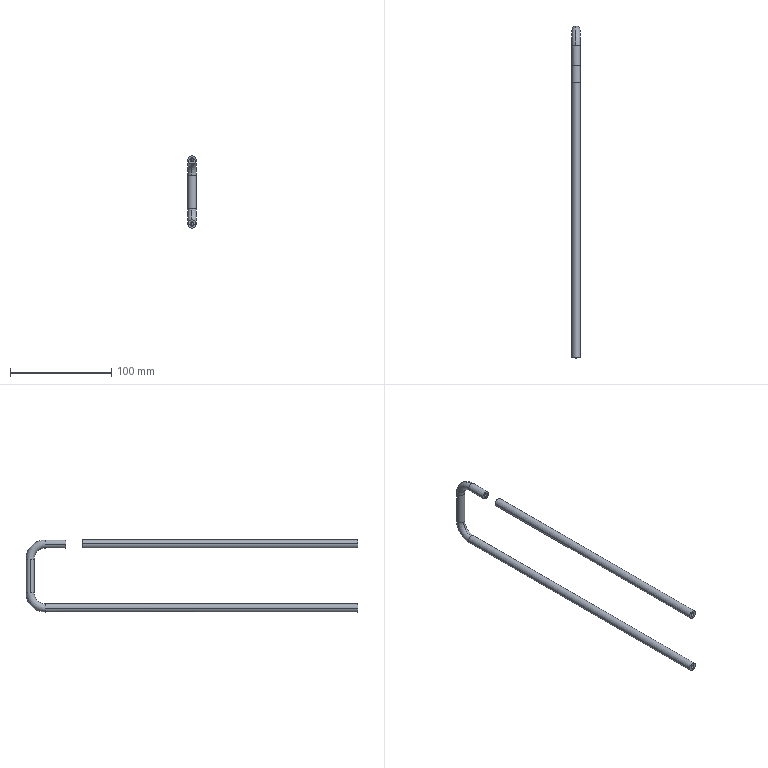Part | SolidWorks | features BaseBody 2 | 2 solids | 28 faces | box 8 x 327.5 x 71.18 mm | volume 25643 mm3 | cylinder 16 | torus 8 | plane 4 | commonest cylinder face diameters 4 x8 8 x8
STEP:
#1=CARTESIAN_POINT('',(168.,-280.,-49.));
#2=VERTEX_POINT('',#1);
#3=CARTESIAN_POINT('',(172.,-280.,-49.));
#4=VERTEX_POINT('',#3);
#5=CARTESIAN_POINT('',(170.,-280.,-49.));
#6=DIRECTION('',(0.,-1.,0.));
#7=DIRECTION('',(-1.,0.,0.));
#8=AXIS2_PLACEMENT_3D('',#5,#6,#7);
#9=CIRCLE('',#8,2.);
#10=EDGE_CURVE('',#2,#4,#9,.T.);
#11=ORIENTED_EDGE('',*,*,#10,.F.);
#12=CARTESIAN_POINT('',(170.,-280.,-49.));
#13=DIRECTION('',(0.,-1.,0.));
#14=DIRECTION('',(1.,0.,0.));
#15=AXIS2_PLACEMENT_3D('',#12,#13,#14);
#16=CIRCLE('',#15,2.);
#17=EDGE_CURVE('',#4,#2,#16,.T.);
#18=ORIENTED_EDGE('',*,*,#17,.F.);
#19=EDGE_LOOP('',(#11,#18));
#20=FACE_BOUND('',#19,.T.);
#21=CARTESIAN_POINT('',(166.,-280.,-49.));
#22=VERTEX_POINT('',#21);
#23=CARTESIAN_POINT('',(174.,-280.,-49.));
#24=VERTEX_POINT('',#23);
#25=CARTESIAN_POINT('',(170.,-280.,-49.));
#26=DIRECTION('',(0.,1.,0.));
#27=DIRECTION('',(-1.,0.,0.));
#28=AXIS2_PLACEMENT_3D('',#25,#26,#27);
#29=CIRCLE('',#28,4.);
#30=EDGE_CURVE('',#22,#24,#29,.T.);
#31=ORIENTED_EDGE('',*,*,#30,.F.);
#32=CARTESIAN_POINT('',(170.,-280.,-49.));
#33=DIRECTION('',(0.,1.,0.));
#34=DIRECTION('',(1.,0.,0.));
#35=AXIS2_PLACEMENT_3D('',#32,#33,#34);
#36=CIRCLE('',#35,4.);
#37=EDGE_CURVE('',#24,#22,#36,.T.);
#38=ORIENTED_EDGE('',*,*,#37,.F.);
#39=EDGE_LOOP('',(#31,#38));
#40=FACE_OUTER_BOUND('',#39,.T.);
#41=CARTESIAN_POINT('',(170.,-280.,-49.));
#42=DIRECTION('',(0.,-1.,0.));
#43=DIRECTION('',(0.,0.,-1.));
#44=AXIS2_PLACEMENT_3D('',#41,#42,#43);
#45=PLANE('',#44);
#46=ADVANCED_FACE('',(#20,#40),#45,.T.);
#47=CARTESIAN_POINT('',(168.,8.5,14.08));
#48=VERTEX_POINT('',#47);
#49=CARTESIAN_POINT('',(172.,8.5,14.08));
#50=VERTEX_POINT('',#49);
#51=CARTESIAN_POINT('',(170.,8.5,14.08));
#52=DIRECTION('',(0.,-1.,0.));
#53=DIRECTION('',(-1.,0.,0.));
#54=AXIS2_PLACEMENT_3D('',#51,#52,#53);
#55=CIRCLE('',#54,2.);
#56=EDGE_CURVE('',#48,#50,#55,.T.);
#57=ORIENTED_EDGE('',*,*,#56,.F.);
#58=CARTESIAN_POINT('',(170.,8.5,14.08));
#59=DIRECTION('',(0.,-1.,0.));
#60=DIRECTION('',(1.,0.,0.));
#61=AXIS2_PLACEMENT_3D('',#58,#59,#60);
#62=CIRCLE('',#61,2.);
#63=EDGE_CURVE('',#50,#48,#62,.T.);
#64=ORIENTED_EDGE('',*,*,#63,.F.);
#65=EDGE_LOOP('',(#57,#64));
#66=FACE_BOUND('',#65,.T.);
#67=CARTESIAN_POINT('',(166.,8.5,14.08));
#68=VERTEX_POINT('',#67);
#69=CARTESIAN_POINT('',(174.,8.5,14.08));
#70=VERTEX_POINT('',#69);
#71=CARTESIAN_POINT('',(170.,8.5,14.08));
#72=DIRECTION('',(0.,1.,0.));
#73=DIRECTION('',(-1.,0.,0.));
#74=AXIS2_PLACEMENT_3D('',#71,#72,#73);
#75=CIRCLE('',#74,4.);
#76=EDGE_CURVE('',#68,#70,#75,.T.);
#77=ORIENTED_EDGE('',*,*,#76,.F.);
#78=CARTESIAN_POINT('',(170.,8.5,14.08));
#79=DIRECTION('',(0.,1.,0.));
#80=DIRECTION('',(1.,0.,0.));
#81=AXIS2_PLACEMENT_3D('',#78,#79,#80);
#82=CIRCLE('',#81,4.);
#83=EDGE_CURVE('',#70,#68,#82,.T.);
#84=ORIENTED_EDGE('',*,*,#83,.F.);
#85=EDGE_LOOP('',(#77,#84));
#86=FACE_OUTER_BOUND('',#85,.T.);
#87=CARTESIAN_POINT('',(170.,8.5,14.08));
#88=DIRECTION('',(0.,-1.,0.));
#89=DIRECTION('',(0.,0.,-1.));
#90=AXIS2_PLACEMENT_3D('',#87,#88,#89);
#91=PLANE('',#90);
#92=ADVANCED_FACE('',(#66,#86),#91,.T.);
#93=CARTESIAN_POINT('',(166.,28.5,-49.));
#94=VERTEX_POINT('',#93);
#95=CARTESIAN_POINT('',(170.,28.5,-45.));
#96=VERTEX_POINT('',#95);
#97=CARTESIAN_POINT('',(170.,28.5,-49.));
#98=DIRECTION('',(0.,1.,0.));
#99=DIRECTION('',(-1.,0.,0.));
#100=AXIS2_PLACEMENT_3D('',#97,#98,#99);
#101=CIRCLE('',#100,4.);
#102=EDGE_CURVE('',#94,#96,#101,.T.);
#103=ORIENTED_EDGE('',*,*,#102,.F.);
#104=CARTESIAN_POINT('',(166.,-280.,-49.));
#105=DIRECTION('',(0.,1.,0.));
#106=VECTOR('',#105,1000.);
#107=LINE('',#104,#106);
#108=EDGE_CURVE('',#22,#94,#107,.T.);
#109=ORIENTED_EDGE('',*,*,#108,.F.);
#110=ORIENTED_EDGE('',*,*,#30,.T.);
#111=CARTESIAN_POINT('',(174.,28.5,-49.));
#112=VERTEX_POINT('',#111);
#113=CARTESIAN_POINT('',(174.,28.5,-49.));
#114=DIRECTION('',(0.,-1.,0.));
#115=VECTOR('',#114,1000.);
#116=LINE('',#113,#115);
#117=EDGE_CURVE('',#112,#24,#116,.T.);
#118=ORIENTED_EDGE('',*,*,#117,.F.);
#119=CARTESIAN_POINT('',(170.,28.5,-49.));
#120=DIRECTION('',(0.,1.,0.));
#121=DIRECTION('',(0.,0.,1.));
#122=AXIS2_PLACEMENT_3D('',#119,#120,#121);
#123=CIRCLE('',#122,4.);
#124=EDGE_CURVE('',#96,#112,#123,.T.);
#125=ORIENTED_EDGE('',*,*,#124,.F.);
#126=EDGE_LOOP('',(#103,#109,#110,#118,#125));
#127=FACE_OUTER_BOUND('',#126,.T.);
#128=CARTESIAN_POINT('',(170.,-280.,-49.));
#129=DIRECTION('',(0.,1.,0.));
#130=DIRECTION('',(-1.,0.,0.));
#131=AXIS2_PLACEMENT_3D('',#128,#129,#130);
#132=CYLINDRICAL_SURFACE('',#131,4.);
#133=ADVANCED_FACE('',(#127),#132,.T.);
#134=ORIENTED_EDGE('',*,*,#117,.T.);
#135=ORIENTED_EDGE('',*,*,#37,.T.);
#136=ORIENTED_EDGE('',*,*,#108,.T.);
#137=CARTESIAN_POINT('',(170.,28.5,-53.));
#138=VERTEX_POINT('',#137);
#139=CARTESIAN_POINT('',(170.,28.5,-49.));
#140=DIRECTION('',(0.,1.,0.));
#141=DIRECTION('',(0.,0.,-1.));
#142=AXIS2_PLACEMENT_3D('',#139,#140,#141);
#143=CIRCLE('',#142,4.);
#144=EDGE_CURVE('',#138,#94,#143,.T.);
#145=ORIENTED_EDGE('',*,*,#144,.F.);
#146=CARTESIAN_POINT('',(170.,28.5,-49.));
#147=DIRECTION('',(0.,-1.,0.));
#148=DIRECTION('',(0.,0.,-1.));
#149=AXIS2_PLACEMENT_3D('',#146,#147,#148);
#150=CIRCLE('',#149,4.);
#151=EDGE_CURVE('',#138,#112,#150,.T.);
#152=ORIENTED_EDGE('',*,*,#151,.T.);
#153=EDGE_LOOP('',(#134,#135,#136,#145,#152));
#154=FACE_OUTER_BOUND('',#153,.T.);
#155=CARTESIAN_POINT('',(170.,-280.,-49.));
#156=DIRECTION('',(0.,1.,0.));
#157=DIRECTION('',(-1.,0.,0.));
#158=AXIS2_PLACEMENT_3D('',#155,#156,#157);
#159=CYLINDRICAL_SURFACE('',#158,4.);
#160=ADVANCED_FACE('',(#154),#159,.T.);
#161=CARTESIAN_POINT('',(170.,39.5,-34.));
#162=VERTEX_POINT('',#161);
#163=CARTESIAN_POINT('',(166.,43.5,-34.));
#164=VERTEX_POINT('',#163);
#165=CARTESIAN_POINT('',(170.,43.5,-34.));
#166=DIRECTION('',(0.,0.,-1.));
#167=DIRECTION('',(0.,-1.,0.));
#168=AXIS2_PLACEMENT_3D('',#165,#166,#167);
#169=CIRCLE('',#168,4.);
#170=EDGE_CURVE('',#162,#164,#169,.T.);
#171=ORIENTED_EDGE('',*,*,#170,.T.);
#172=CARTESIAN_POINT('',(170.,47.5,-34.));
#173=VERTEX_POINT('',#172);
#174=CARTESIAN_POINT('',(170.,43.5,-34.));
#175=DIRECTION('',(0.,0.,-1.));
#176=DIRECTION('',(-1.,0.,0.));
#177=AXIS2_PLACEMENT_3D('',#174,#175,#176);
#178=CIRCLE('',#177,4.);
#179=EDGE_CURVE('',#164,#173,#178,.T.);
#180=ORIENTED_EDGE('',*,*,#179,.T.);
#181=CARTESIAN_POINT('',(170.,28.5,-34.));
#182=DIRECTION('',(1.,0.,0.));
#183=DIRECTION('',(0.,0.,-1.));
#184=AXIS2_PLACEMENT_3D('',#181,#182,#183);
#185=CIRCLE('',#184,19.);
#186=EDGE_CURVE('',#138,#173,#185,.T.);
#187=ORIENTED_EDGE('',*,*,#186,.F.);
#188=ORIENTED_EDGE('',*,*,#144,.T.);
#189=ORIENTED_EDGE('',*,*,#102,.T.);
#190=CARTESIAN_POINT('',(170.,28.5,-34.));
#191=DIRECTION('',(-1.,0.,0.));
#192=DIRECTION('',(0.,1.,0.));
#193=AXIS2_PLACEMENT_3D('',#190,#191,#192);
#194=CIRCLE('',#193,11.);
#195=EDGE_CURVE('',#162,#96,#194,.T.);
#196=ORIENTED_EDGE('',*,*,#195,.F.);
#197=EDGE_LOOP('',(#171,#180,#187,#188,#189,#196));
#198=FACE_OUTER_BOUND('',#197,.T.);
#199=CARTESIAN_POINT('',(170.,28.5,-34.));
#200=DIRECTION('',(-1.,0.,0.));
#201=DIRECTION('',(0.,0.,-1.));
#202=AXIS2_PLACEMENT_3D('',#199,#200,#201);
#203=TOROIDAL_SURFACE('',#202,15.,4.);
#204=ADVANCED_FACE('',(#198),#203,.T.);
#205=CARTESIAN_POINT('',(174.,43.5,-34.));
#206=VERTEX_POINT('',#205);
#207=CARTESIAN_POINT('',(170.,43.5,-34.));
#208=DIRECTION('',(0.,0.,1.));
#209=DIRECTION('',(0.,-1.,0.));
#210=AXIS2_PLACEMENT_3D('',#207,#208,#209);
#211=CIRCLE('',#210,4.);
#212=EDGE_CURVE('',#162,#206,#211,.T.);
#213=ORIENTED_EDGE('',*,*,#212,.F.);
#214=ORIENTED_EDGE('',*,*,#195,.T.);
#215=ORIENTED_EDGE('',*,*,#124,.T.);
#216=ORIENTED_EDGE('',*,*,#151,.F.);
#217=ORIENTED_EDGE('',*,*,#186,.T.);
#218=CARTESIAN_POINT('',(170.,43.5,-34.));
#219=DIRECTION('',(0.,0.,1.));
#220=DIRECTION('',(1.,0.,0.));
#221=AXIS2_PLACEMENT_3D('',#218,#219,#220);
#222=CIRCLE('',#221,4.);
#223=EDGE_CURVE('',#206,#173,#222,.T.);
#224=ORIENTED_EDGE('',*,*,#223,.F.);
#225=EDGE_LOOP('',(#213,#214,#215,#216,#217,#224));
#226=FACE_OUTER_BOUND('',#225,.T.);
#227=CARTESIAN_POINT('',(170.,28.5,-34.));
#228=DIRECTION('',(-1.,0.,0.));
#229=DIRECTION('',(0.,0.,-1.));
#230=AXIS2_PLACEMENT_3D('',#227,#228,#229);
#231=TOROIDAL_SURFACE('',#230,15.,4.);
#232=ADVANCED_FACE('',(#226),#231,.T.);
#233=CARTESIAN_POINT('',(166.,43.5,-0.92));
#234=VERTEX_POINT('',#233);
#235=CARTESIAN_POINT('',(170.,39.5,-0.92));
#236=VERTEX_POINT('',#235);
#237=CARTESIAN_POINT('',(170.,43.5,-0.92));
#238=DIRECTION('',(0.,0.,1.));
#239=DIRECTION('',(-1.,0.,0.));
#240=AXIS2_PLACEMENT_3D('',#237,#238,#239);
#241=CIRCLE('',#240,4.);
#242=EDGE_CURVE('',#234,#236,#241,.T.);
#243=ORIENTED_EDGE('',*,*,#242,.F.);
#244=CARTESIAN_POINT('',(166.,43.5,-34.));
#245=DIRECTION('',(0.,0.,1.));
#246=VECTOR('',#245,1000.);
#247=LINE('',#244,#246);
#248=EDGE_CURVE('',#164,#234,#247,.T.);
#249=ORIENTED_EDGE('',*,*,#248,.F.);
#250=ORIENTED_EDGE('',*,*,#170,.F.);
#251=ORIENTED_EDGE('',*,*,#212,.T.);
#252=CARTESIAN_POINT('',(174.,43.5,-0.92));
#253=VERTEX_POINT('',#252);
#254=CARTESIAN_POINT('',(174.,43.5,-0.92));
#255=DIRECTION('',(0.,0.,-1.));
#256=VECTOR('',#255,1000.);
#257=LINE('',#254,#256);
#258=EDGE_CURVE('',#253,#206,#257,.T.);
#259=ORIENTED_EDGE('',*,*,#258,.F.);
#260=CARTESIAN_POINT('',(170.,43.5,-0.92));
#261=DIRECTION('',(0.,0.,1.));
#262=DIRECTION('',(0.,-1.,0.));
#263=AXIS2_PLACEMENT_3D('',#260,#261,#262);
#264=CIRCLE('',#263,4.);
#265=EDGE_CURVE('',#236,#253,#264,.T.);
#266=ORIENTED_EDGE('',*,*,#265,.F.);
#267=EDGE_LOOP('',(#243,#249,#250,#251,#259,#266));
#268=FACE_OUTER_BOUND('',#267,.T.);
#269=CARTESIAN_POINT('',(170.,43.5,-34.));
#270=DIRECTION('',(0.,0.,1.));
#271=DIRECTION('',(-1.,0.,0.));
#272=AXIS2_PLACEMENT_3D('',#269,#270,#271);
#273=CYLINDRICAL_SURFACE('',#272,4.);
#274=ADVANCED_FACE('',(#268),#273,.T.);
#275=ORIENTED_EDGE('',*,*,#258,.T.);
#276=ORIENTED_EDGE('',*,*,#223,.T.);
#277=ORIENTED_EDGE('',*,*,#179,.F.);
#278=ORIENTED_EDGE('',*,*,#248,.T.);
#279=CARTESIAN_POINT('',(170.,47.5,-0.92));
#280=VERTEX_POINT('',#279);
#281=CARTESIAN_POINT('',(170.,43.5,-0.92));
#282=DIRECTION('',(0.,0.,1.));
#283=DIRECTION('',(0.,1.,0.));
#284=AXIS2_PLACEMENT_3D('',#281,#282,#283);
#285=CIRCLE('',#284,4.);
#286=EDGE_CURVE('',#280,#234,#285,.T.);
#287=ORIENTED_EDGE('',*,*,#286,.F.);
#288=CARTESIAN_POINT('',(170.,43.5,-0.92));
#289=DIRECTION('',(0.,0.,-1.));
#290=DIRECTION('',(0.,1.,0.));
#291=AXIS2_PLACEMENT_3D('',#288,#289,#290);
#292=CIRCLE('',#291,4.);
#293=EDGE_CURVE('',#280,#253,#292,.T.);
#294=ORIENTED_EDGE('',*,*,#293,.T.);
#295=EDGE_LOOP('',(#275,#276,#277,#278,#287,#294));
#296=FACE_OUTER_BOUND('',#295,.T.);
#297=CARTESIAN_POINT('',(170.,43.5,-34.));
#298=DIRECTION('',(0.,0.,1.));
#299=DIRECTION('',(-1.,0.,0.));
#300=AXIS2_PLACEMENT_3D('',#297,#298,#299);
#301=CYLINDRICAL_SURFACE('',#300,4.);
#302=ADVANCED_FACE('',(#296),#301,.T.);
#303=CARTESIAN_POINT('',(170.,28.5,10.08));
#304=VERTEX_POINT('',#303);
#305=CARTESIAN_POINT('',(166.,28.5,14.08));
#306=VERTEX_POINT('',#305);
#307=CARTESIAN_POINT('',(170.,28.5,14.08));
#308=DIRECTION('',(0.,1.,0.));
#309=DIRECTION('',(0.,0.,-1.));
#310=AXIS2_PLACEMENT_3D('',#307,#308,#309);
#311=CIRCLE('',#310,4.);
#312=EDGE_CURVE('',#304,#306,#311,.T.);
#313=ORIENTED_EDGE('',*,*,#312,.T.);
#314=CARTESIAN_POINT('',(170.,28.5,18.08));
#315=VERTEX_POINT('',#314);
#316=CARTESIAN_POINT('',(170.,28.5,14.08));
#317=DIRECTION('',(0.,1.,0.));
#318=DIRECTION('',(-1.,0.,0.));
#319=AXIS2_PLACEMENT_3D('',#316,#317,#318);
#320=CIRCLE('',#319,4.);
#321=EDGE_CURVE('',#306,#315,#320,.T.);
#322=ORIENTED_EDGE('',*,*,#321,.T.);
#323=CARTESIAN_POINT('',(170.,28.5,-0.92));
#324=DIRECTION('',(1.,0.,0.));
#325=DIRECTION('',(0.,1.,0.));
#326=AXIS2_PLACEMENT_3D('',#323,#324,#325);
#327=CIRCLE('',#326,19.);
#328=EDGE_CURVE('',#280,#315,#327,.T.);
#329=ORIENTED_EDGE('',*,*,#328,.F.);
#330=ORIENTED_EDGE('',*,*,#286,.T.);
#331=ORIENTED_EDGE('',*,*,#242,.T.);
#332=CARTESIAN_POINT('',(170.,28.5,-0.92));
#333=DIRECTION('',(-1.,0.,0.));
#334=DIRECTION('',(0.,0.,1.));
#335=AXIS2_PLACEMENT_3D('',#332,#333,#334);
#336=CIRCLE('',#335,11.);
#337=EDGE_CURVE('',#304,#236,#336,.T.);
#338=ORIENTED_EDGE('',*,*,#337,.F.);
#339=EDGE_LOOP('',(#313,#322,#329,#330,#331,#338));
#340=FACE_OUTER_BOUND('',#339,.T.);
#341=CARTESIAN_POINT('',(170.,28.5,-0.92));
#342=DIRECTION('',(-1.,0.,0.));
#343=DIRECTION('',(0.,1.,0.));
#344=AXIS2_PLACEMENT_3D('',#341,#342,#343);
#345=TOROIDAL_SURFACE('',#344,15.,4.);
#346=ADVANCED_FACE('',(#340),#345,.T.);
#347=CARTESIAN_POINT('',(174.,28.5,14.08));
#348=VERTEX_POINT('',#347);
#349=CARTESIAN_POINT('',(170.,28.5,14.08));
#350=DIRECTION('',(0.,-1.,0.));
#351=DIRECTION('',(0.,0.,-1.));
#352=AXIS2_PLACEMENT_3D('',#349,#350,#351);
#353=CIRCLE('',#352,4.);
#354=EDGE_CURVE('',#304,#348,#353,.T.);
#355=ORIENTED_EDGE('',*,*,#354,.F.);
#356=ORIENTED_EDGE('',*,*,#337,.T.);
#357=ORIENTED_EDGE('',*,*,#265,.T.);
#358=ORIENTED_EDGE('',*,*,#293,.F.);
#359=ORIENTED_EDGE('',*,*,#328,.T.);
#360=CARTESIAN_POINT('',(170.,28.5,14.08));
#361=DIRECTION('',(0.,-1.,0.));
#362=DIRECTION('',(1.,0.,0.));
#363=AXIS2_PLACEMENT_3D('',#360,#361,#362);
#364=CIRCLE('',#363,4.);
#365=EDGE_CURVE('',#348,#315,#364,.T.);
#366=ORIENTED_EDGE('',*,*,#365,.F.);
#367=EDGE_LOOP('',(#355,#356,#357,#358,#359,#366));
#368=FACE_OUTER_BOUND('',#367,.T.);
#369=CARTESIAN_POINT('',(170.,28.5,-0.92));
#370=DIRECTION('',(-1.,0.,0.));
#371=DIRECTION('',(0.,1.,0.));
#372=AXIS2_PLACEMENT_3D('',#369,#370,#371);
#373=TOROIDAL_SURFACE('',#372,15.,4.);
#374=ADVANCED_FACE('',(#368),#373,.T.);
#375=ORIENTED_EDGE('',*,*,#83,.T.);
#376=CARTESIAN_POINT('',(166.,28.5,14.08));
#377=DIRECTION('',(0.,-1.,0.));
#378=VECTOR('',#377,1000.);
#379=LINE('',#376,#378);
#380=EDGE_CURVE('',#306,#68,#379,.T.);
#381=ORIENTED_EDGE('',*,*,#380,.F.);
#382=ORIENTED_EDGE('',*,*,#312,.F.);
#383=ORIENTED_EDGE('',*,*,#354,.T.);
#384=CARTESIAN_POINT('',(174.,8.5,14.08));
#385=DIRECTION('',(0.,1.,0.));
#386=VECTOR('',#385,1000.);
#387=LINE('',#384,#386);
#388=EDGE_CURVE('',#70,#348,#387,.T.);
#389=ORIENTED_EDGE('',*,*,#388,.F.);
#390=EDGE_LOOP('',(#375,#381,#382,#383,#389));
#391=FACE_OUTER_BOUND('',#390,.T.);
#392=CARTESIAN_POINT('',(170.,28.5,14.08));
#393=DIRECTION('',(0.,-1.,0.));
#394=DIRECTION('',(-1.,0.,0.));
#395=AXIS2_PLACEMENT_3D('',#392,#393,#394);
#396=CYLINDRICAL_SURFACE('',#395,4.);
#397=ADVANCED_FACE('',(#391),#396,.T.);
#398=ORIENTED_EDGE('',*,*,#388,.T.);
#399=ORIENTED_EDGE('',*,*,#365,.T.);
#400=ORIENTED_EDGE('',*,*,#321,.F.);
#401=ORIENTED_EDGE('',*,*,#380,.T.);
#402=ORIENTED_EDGE('',*,*,#76,.T.);
#403=EDGE_LOOP('',(#398,#399,#400,#401,#402));
#404=FACE_OUTER_BOUND('',#403,.T.);
#405=CARTESIAN_POINT('',(170.,28.5,14.08));
#406=DIRECTION('',(0.,-1.,0.));
#407=DIRECTION('',(-1.,0.,0.));
#408=AXIS2_PLACEMENT_3D('',#405,#406,#407);
#409=CYLINDRICAL_SURFACE('',#408,4.);
#410=ADVANCED_FACE('',(#404),#409,.T.);
#411=ORIENTED_EDGE('',*,*,#17,.T.);
#412=CARTESIAN_POINT('',(168.,28.5,-49.));
#413=VERTEX_POINT('',#412);
#414=CARTESIAN_POINT('',(168.,28.5,-49.));
#415=DIRECTION('',(0.,-1.,0.));
#416=VECTOR('',#415,1000.);
#417=LINE('',#414,#416);
#418=EDGE_CURVE('',#413,#2,#417,.T.);
#419=ORIENTED_EDGE('',*,*,#418,.F.);
#420=CARTESIAN_POINT('',(170.,28.5,-47.));
#421=VERTEX_POINT('',#420);
#422=CARTESIAN_POINT('',(170.,28.5,-49.));
#423=DIRECTION('',(0.,-1.,0.));
#424=DIRECTION('',(0.,0.,1.));
#425=AXIS2_PLACEMENT_3D('',#422,#423,#424);
#426=CIRCLE('',#425,2.);
#427=EDGE_CURVE('',#421,#413,#426,.T.);
#428=ORIENTED_EDGE('',*,*,#427,.F.);
#429=CARTESIAN_POINT('',(172.,28.5,-49.));
#430=VERTEX_POINT('',#429);
#431=CARTESIAN_POINT('',(170.,28.5,-49.));
#432=DIRECTION('',(0.,-1.,0.));
#433=DIRECTION('',(1.,0.,0.));
#434=AXIS2_PLACEMENT_3D('',#431,#432,#433);
#435=CIRCLE('',#434,2.);
#436=EDGE_CURVE('',#430,#421,#435,.T.);
#437=ORIENTED_EDGE('',*,*,#436,.F.);
#438=CARTESIAN_POINT('',(172.,-280.,-49.));
#439=DIRECTION('',(0.,1.,0.));
#440=VECTOR('',#439,1000.);
#441=LINE('',#438,#440);
#442=EDGE_CURVE('',#4,#430,#441,.T.);
#443=ORIENTED_EDGE('',*,*,#442,.F.);
#444=EDGE_LOOP('',(#411,#419,#428,#437,#443));
#445=FACE_OUTER_BOUND('',#444,.T.);
#446=CARTESIAN_POINT('',(170.,-280.,-49.));
#447=DIRECTION('',(0.,1.,0.));
#448=DIRECTION('',(-1.,0.,0.));
#449=AXIS2_PLACEMENT_3D('',#446,#447,#448);
#450=CYLINDRICAL_SURFACE('',#449,2.);
#451=ADVANCED_FACE('',(#445),#450,.F.);
#452=ORIENTED_EDGE('',*,*,#442,.T.);
#453=CARTESIAN_POINT('',(170.,28.5,-51.));
#454=VERTEX_POINT('',#453);
#455=CARTESIAN_POINT('',(170.,28.5,-49.));
#456=DIRECTION('',(0.,1.,0.));
#457=DIRECTION('',(1.,0.,0.));
#458=AXIS2_PLACEMENT_3D('',#455,#456,#457);
#459=CIRCLE('',#458,2.);
#460=EDGE_CURVE('',#430,#454,#459,.T.);
#461=ORIENTED_EDGE('',*,*,#460,.T.);
#462=CARTESIAN_POINT('',(170.,28.5,-49.));
#463=DIRECTION('',(0.,1.,0.));
#464=DIRECTION('',(0.,0.,-1.));
#465=AXIS2_PLACEMENT_3D('',#462,#463,#464);
#466=CIRCLE('',#465,2.);
#467=EDGE_CURVE('',#454,#413,#466,.T.);
#468=ORIENTED_EDGE('',*,*,#467,.T.);
#469=ORIENTED_EDGE('',*,*,#418,.T.);
#470=ORIENTED_EDGE('',*,*,#10,.T.);
#471=EDGE_LOOP('',(#452,#461,#468,#469,#470));
#472=FACE_OUTER_BOUND('',#471,.T.);
#473=CARTESIAN_POINT('',(170.,-280.,-49.));
#474=DIRECTION('',(0.,1.,0.));
#475=DIRECTION('',(-1.,0.,0.));
#476=AXIS2_PLACEMENT_3D('',#473,#474,#475);
#477=CYLINDRICAL_SURFACE('',#476,2.);
#478=ADVANCED_FACE('',(#472),#477,.F.);
#479=ORIENTED_EDGE('',*,*,#427,.T.);
#480=ORIENTED_EDGE('',*,*,#467,.F.);
#481=CARTESIAN_POINT('',(170.,45.5,-34.));
#482=VERTEX_POINT('',#481);
#483=CARTESIAN_POINT('',(170.,28.5,-34.));
#484=DIRECTION('',(-1.,0.,0.));
#485=DIRECTION('',(0.,1.,0.));
#486=AXIS2_PLACEMENT_3D('',#483,#484,#485);
#487=CIRCLE('',#486,17.);
#488=EDGE_CURVE('',#482,#454,#487,.T.);
#489=ORIENTED_EDGE('',*,*,#488,.F.);
#490=CARTESIAN_POINT('',(168.,43.5,-34.));
#491=VERTEX_POINT('',#490);
#492=CARTESIAN_POINT('',(170.,43.5,-34.));
#493=DIRECTION('',(0.,0.,-1.));
#494=DIRECTION('',(-1.,0.,0.));
#495=AXIS2_PLACEMENT_3D('',#492,#493,#494);
#496=CIRCLE('',#495,2.);
#497=EDGE_CURVE('',#491,#482,#496,.T.);
#498=ORIENTED_EDGE('',*,*,#497,.F.);
#499=CARTESIAN_POINT('',(170.,41.5,-34.));
#500=VERTEX_POINT('',#499);
#501=CARTESIAN_POINT('',(170.,43.5,-34.));
#502=DIRECTION('',(0.,0.,1.));
#503=DIRECTION('',(-1.,0.,0.));
#504=AXIS2_PLACEMENT_3D('',#501,#502,#503);
#505=CIRCLE('',#504,2.);
#506=EDGE_CURVE('',#491,#500,#505,.T.);
#507=ORIENTED_EDGE('',*,*,#506,.T.);
#508=CARTESIAN_POINT('',(170.,28.5,-34.));
#509=DIRECTION('',(1.,0.,0.));
#510=DIRECTION('',(0.,0.,-1.));
#511=AXIS2_PLACEMENT_3D('',#508,#509,#510);
#512=CIRCLE('',#511,13.);
#513=EDGE_CURVE('',#421,#500,#512,.T.);
#514=ORIENTED_EDGE('',*,*,#513,.F.);
#515=EDGE_LOOP('',(#479,#480,#489,#498,#507,#514));
#516=FACE_OUTER_BOUND('',#515,.T.);
#517=CARTESIAN_POINT('',(170.,28.5,-34.));
#518=DIRECTION('',(1.,0.,0.));
#519=DIRECTION('',(0.,1.,0.));
#520=AXIS2_PLACEMENT_3D('',#517,#518,#519);
#521=TOROIDAL_SURFACE('',#520,15.,2.);
#522=ADVANCED_FACE('',(#516),#521,.F.);
#523=ORIENTED_EDGE('',*,*,#436,.T.);
#524=ORIENTED_EDGE('',*,*,#513,.T.);
#525=CARTESIAN_POINT('',(172.,43.5,-34.));
#526=VERTEX_POINT('',#525);
#527=CARTESIAN_POINT('',(170.,43.5,-34.));
#528=DIRECTION('',(0.,0.,-1.));
#529=DIRECTION('',(1.,0.,0.));
#530=AXIS2_PLACEMENT_3D('',#527,#528,#529);
#531=CIRCLE('',#530,2.);
#532=EDGE_CURVE('',#526,#500,#531,.T.);
#533=ORIENTED_EDGE('',*,*,#532,.F.);
#534=CARTESIAN_POINT('',(170.,43.5,-34.));
#535=DIRECTION('',(0.,0.,-1.));
#536=DIRECTION('',(0.,1.,0.));
#537=AXIS2_PLACEMENT_3D('',#534,#535,#536);
#538=CIRCLE('',#537,2.);
#539=EDGE_CURVE('',#482,#526,#538,.T.);
#540=ORIENTED_EDGE('',*,*,#539,.F.);
#541=ORIENTED_EDGE('',*,*,#488,.T.);
#542=ORIENTED_EDGE('',*,*,#460,.F.);
#543=EDGE_LOOP('',(#523,#524,#533,#540,#541,#542));
#544=FACE_OUTER_BOUND('',#543,.T.);
#545=CARTESIAN_POINT('',(170.,28.5,-34.));
#546=DIRECTION('',(1.,0.,0.));
#547=DIRECTION('',(0.,1.,0.));
#548=AXIS2_PLACEMENT_3D('',#545,#546,#547);
#549=TOROIDAL_SURFACE('',#548,15.,2.);
#550=ADVANCED_FACE('',(#544),#549,.F.);
#551=ORIENTED_EDGE('',*,*,#506,.F.);
#552=CARTESIAN_POINT('',(168.,43.5,-0.92));
#553=VERTEX_POINT('',#552);
#554=CARTESIAN_POINT('',(168.,43.5,-0.92));
#555=DIRECTION('',(0.,0.,-1.));
#556=VECTOR('',#555,1000.);
#557=LINE('',#554,#556);
#558=EDGE_CURVE('',#553,#491,#557,.T.);
#559=ORIENTED_EDGE('',*,*,#558,.F.);
#560=CARTESIAN_POINT('',(170.,41.5,-0.92));
#561=VERTEX_POINT('',#560);
#562=CARTESIAN_POINT('',(170.,43.5,-0.92));
#563=DIRECTION('',(0.,0.,-1.));
#564=DIRECTION('',(0.,-1.,0.));
#565=AXIS2_PLACEMENT_3D('',#562,#563,#564);
#566=CIRCLE('',#565,2.);
#567=EDGE_CURVE('',#561,#553,#566,.T.);
#568=ORIENTED_EDGE('',*,*,#567,.F.);
#569=CARTESIAN_POINT('',(172.,43.5,-0.92));
#570=VERTEX_POINT('',#569);
#571=CARTESIAN_POINT('',(170.,43.5,-0.92));
#572=DIRECTION('',(0.,0.,-1.));
#573=DIRECTION('',(1.,0.,0.));
#574=AXIS2_PLACEMENT_3D('',#571,#572,#573);
#575=CIRCLE('',#574,2.);
#576=EDGE_CURVE('',#570,#561,#575,.T.);
#577=ORIENTED_EDGE('',*,*,#576,.F.);
#578=CARTESIAN_POINT('',(172.,43.5,-34.));
#579=DIRECTION('',(0.,0.,1.));
#580=VECTOR('',#579,1000.);
#581=LINE('',#578,#580);
#582=EDGE_CURVE('',#526,#570,#581,.T.);
#583=ORIENTED_EDGE('',*,*,#582,.F.);
#584=ORIENTED_EDGE('',*,*,#532,.T.);
#585=EDGE_LOOP('',(#551,#559,#568,#577,#583,#584));
#586=FACE_OUTER_BOUND('',#585,.T.);
#587=CARTESIAN_POINT('',(170.,43.5,-34.));
#588=DIRECTION('',(0.,0.,1.));
#589=DIRECTION('',(-1.,0.,0.));
#590=AXIS2_PLACEMENT_3D('',#587,#588,#589);
#591=CYLINDRICAL_SURFACE('',#590,2.);
#592=ADVANCED_FACE('',(#586),#591,.F.);
#593=ORIENTED_EDGE('',*,*,#582,.T.);
#594=CARTESIAN_POINT('',(170.,45.5,-0.92));
#595=VERTEX_POINT('',#594);
#596=CARTESIAN_POINT('',(170.,43.5,-0.92));
#597=DIRECTION('',(0.,0.,1.));
#598=DIRECTION('',(1.,0.,0.));
#599=AXIS2_PLACEMENT_3D('',#596,#597,#598);
#600=CIRCLE('',#599,2.);
#601=EDGE_CURVE('',#570,#595,#600,.T.);
#602=ORIENTED_EDGE('',*,*,#601,.T.);
#603=CARTESIAN_POINT('',(170.,43.5,-0.92));
#604=DIRECTION('',(0.,0.,1.));
#605=DIRECTION('',(0.,1.,0.));
#606=AXIS2_PLACEMENT_3D('',#603,#604,#605);
#607=CIRCLE('',#606,2.);
#608=EDGE_CURVE('',#595,#553,#607,.T.);
#609=ORIENTED_EDGE('',*,*,#608,.T.);
#610=ORIENTED_EDGE('',*,*,#558,.T.);
#611=ORIENTED_EDGE('',*,*,#497,.T.);
#612=ORIENTED_EDGE('',*,*,#539,.T.);
#613=EDGE_LOOP('',(#593,#602,#609,#610,#611,#612));
#614=FACE_OUTER_BOUND('',#613,.T.);
#615=CARTESIAN_POINT('',(170.,43.5,-34.));
#616=DIRECTION('',(0.,0.,1.));
#617=DIRECTION('',(-1.,0.,0.));
#618=AXIS2_PLACEMENT_3D('',#615,#616,#617);
#619=CYLINDRICAL_SURFACE('',#618,2.);
#620=ADVANCED_FACE('',(#614),#619,.F.);
#621=ORIENTED_EDGE('',*,*,#567,.T.);
#622=ORIENTED_EDGE('',*,*,#608,.F.);
#623=CARTESIAN_POINT('',(170.,28.5,16.08));
#624=VERTEX_POINT('',#623);
#625=CARTESIAN_POINT('',(170.,28.5,-0.92));
#626=DIRECTION('',(-1.,0.,0.));
#627=DIRECTION('',(0.,0.,1.));
#628=AXIS2_PLACEMENT_3D('',#625,#626,#627);
#629=CIRCLE('',#628,17.);
#630=EDGE_CURVE('',#624,#595,#629,.T.);
#631=ORIENTED_EDGE('',*,*,#630,.F.);
#632=CARTESIAN_POINT('',(168.,28.5,14.08));
#633=VERTEX_POINT('',#632);
#634=CARTESIAN_POINT('',(170.,28.5,14.08));
#635=DIRECTION('',(0.,1.,0.));
#636=DIRECTION('',(-1.,0.,0.));
#637=AXIS2_PLACEMENT_3D('',#634,#635,#636);
#638=CIRCLE('',#637,2.);
#639=EDGE_CURVE('',#633,#624,#638,.T.);
#640=ORIENTED_EDGE('',*,*,#639,.F.);
#641=CARTESIAN_POINT('',(170.,28.5,12.08));
#642=VERTEX_POINT('',#641);
#643=CARTESIAN_POINT('',(170.,28.5,14.08));
#644=DIRECTION('',(0.,-1.,0.));
#645=DIRECTION('',(-1.,0.,0.));
#646=AXIS2_PLACEMENT_3D('',#643,#644,#645);
#647=CIRCLE('',#646,2.);
#648=EDGE_CURVE('',#633,#642,#647,.T.);
#649=ORIENTED_EDGE('',*,*,#648,.T.);
#650=CARTESIAN_POINT('',(170.,28.5,-0.92));
#651=DIRECTION('',(1.,0.,0.));
#652=DIRECTION('',(0.,1.,0.));
#653=AXIS2_PLACEMENT_3D('',#650,#651,#652);
#654=CIRCLE('',#653,13.);
#655=EDGE_CURVE('',#561,#642,#654,.T.);
#656=ORIENTED_EDGE('',*,*,#655,.F.);
#657=EDGE_LOOP('',(#621,#622,#631,#640,#649,#656));
#658=FACE_OUTER_BOUND('',#657,.T.);
#659=CARTESIAN_POINT('',(170.,28.5,-0.92));
#660=DIRECTION('',(1.,0.,0.));
#661=DIRECTION('',(0.,0.,1.));
#662=AXIS2_PLACEMENT_3D('',#659,#660,#661);
#663=TOROIDAL_SURFACE('',#662,15.,2.);
#664=ADVANCED_FACE('',(#658),#663,.F.);
#665=ORIENTED_EDGE('',*,*,#576,.T.);
#666=ORIENTED_EDGE('',*,*,#655,.T.);
#667=CARTESIAN_POINT('',(172.,28.5,14.08));
#668=VERTEX_POINT('',#667);
#669=CARTESIAN_POINT('',(170.,28.5,14.08));
#670=DIRECTION('',(0.,1.,0.));
#671=DIRECTION('',(1.,0.,0.));
#672=AXIS2_PLACEMENT_3D('',#669,#670,#671);
#673=CIRCLE('',#672,2.);
#674=EDGE_CURVE('',#668,#642,#673,.T.);
#675=ORIENTED_EDGE('',*,*,#674,.F.);
#676=CARTESIAN_POINT('',(170.,28.5,14.08));
#677=DIRECTION('',(0.,1.,0.));
#678=DIRECTION('',(0.,0.,1.));
#679=AXIS2_PLACEMENT_3D('',#676,#677,#678);
#680=CIRCLE('',#679,2.);
#681=EDGE_CURVE('',#624,#668,#680,.T.);
#682=ORIENTED_EDGE('',*,*,#681,.F.);
#683=ORIENTED_EDGE('',*,*,#630,.T.);
#684=ORIENTED_EDGE('',*,*,#601,.F.);
#685=EDGE_LOOP('',(#665,#666,#675,#682,#683,#684));
#686=FACE_OUTER_BOUND('',#685,.T.);
#687=CARTESIAN_POINT('',(170.,28.5,-0.92));
#688=DIRECTION('',(1.,0.,0.));
#689=DIRECTION('',(0.,0.,1.));
#690=AXIS2_PLACEMENT_3D('',#687,#688,#689);
#691=TOROIDAL_SURFACE('',#690,15.,2.);
#692=ADVANCED_FACE('',(#686),#691,.F.);
#693=ORIENTED_EDGE('',*,*,#648,.F.);
#694=CARTESIAN_POINT('',(168.,8.5,14.08));
#695=DIRECTION('',(0.,1.,0.));
#696=VECTOR('',#695,1000.);
#697=LINE('',#694,#696);
#698=EDGE_CURVE('',#48,#633,#697,.T.);
#699=ORIENTED_EDGE('',*,*,#698,.F.);
#700=ORIENTED_EDGE('',*,*,#56,.T.);
#701=CARTESIAN_POINT('',(172.,28.5,14.08));
#702=DIRECTION('',(0.,-1.,0.));
#703=VECTOR('',#702,1000.);
#704=LINE('',#701,#703);
#705=EDGE_CURVE('',#668,#50,#704,.T.);
#706=ORIENTED_EDGE('',*,*,#705,.F.);
#707=ORIENTED_EDGE('',*,*,#674,.T.);
#708=EDGE_LOOP('',(#693,#699,#700,#706,#707));
#709=FACE_OUTER_BOUND('',#708,.T.);
#710=CARTESIAN_POINT('',(170.,28.5,14.08));
#711=DIRECTION('',(0.,-1.,0.));
#712=DIRECTION('',(-1.,0.,0.));
#713=AXIS2_PLACEMENT_3D('',#710,#711,#712);
#714=CYLINDRICAL_SURFACE('',#713,2.);
#715=ADVANCED_FACE('',(#709),#714,.F.);
#716=ORIENTED_EDGE('',*,*,#705,.T.);
#717=ORIENTED_EDGE('',*,*,#63,.T.);
#718=ORIENTED_EDGE('',*,*,#698,.T.);
#719=ORIENTED_EDGE('',*,*,#639,.T.);
#720=ORIENTED_EDGE('',*,*,#681,.T.);
#721=EDGE_LOOP('',(#716,#717,#718,#719,#720));
#722=FACE_OUTER_BOUND('',#721,.T.);
#723=CARTESIAN_POINT('',(170.,28.5,14.08));
#724=DIRECTION('',(0.,-1.,0.));
#725=DIRECTION('',(-1.,0.,0.));
#726=AXIS2_PLACEMENT_3D('',#723,#724,#725);
#727=CYLINDRICAL_SURFACE('',#726,2.);
#728=ADVANCED_FACE('',(#722),#727,.F.);
#729=CLOSED_SHELL('',(#46,#92,#133,#160,#204,#232,#274,#302,#346,#374,#397,#410,#451,#478,#522,#550,#592,#620,#664,#692,#715,#728));
#730=MANIFOLD_SOLID_BREP('',#729);
#731=CARTESIAN_POINT('',(172.,-8.5,14.18));
#732=VERTEX_POINT('',#731);
#733=CARTESIAN_POINT('',(168.,-8.5,14.18));
#734=VERTEX_POINT('',#733);
#735=CARTESIAN_POINT('',(170.,-8.5,14.18));
#736=DIRECTION('',(0.,1.,0.));
#737=DIRECTION('',(1.,0.,0.));
#738=AXIS2_PLACEMENT_3D('',#735,#736,#737);
#739=CIRCLE('',#738,2.);
#740=EDGE_CURVE('',#732,#734,#739,.T.);
#741=ORIENTED_EDGE('',*,*,#740,.F.);
#742=CARTESIAN_POINT('',(170.,-8.5,14.18));
#743=DIRECTION('',(0.,1.,0.));
#744=DIRECTION('',(-1.,0.,0.));
#745=AXIS2_PLACEMENT_3D('',#742,#743,#744);
#746=CIRCLE('',#745,2.);
#747=EDGE_CURVE('',#734,#732,#746,.T.);
#748=ORIENTED_EDGE('',*,*,#747,.F.);
#749=EDGE_LOOP('',(#741,#748));
#750=FACE_BOUND('',#749,.T.);
#751=CARTESIAN_POINT('',(174.,-8.5,14.18));
#752=VERTEX_POINT('',#751);
#753=CARTESIAN_POINT('',(166.,-8.5,14.18));
#754=VERTEX_POINT('',#753);
#755=CARTESIAN_POINT('',(170.,-8.5,14.18));
#756=DIRECTION('',(0.,-1.,0.));
#757=DIRECTION('',(1.,0.,0.));
#758=AXIS2_PLACEMENT_3D('',#755,#756,#757);
#759=CIRCLE('',#758,4.);
#760=EDGE_CURVE('',#752,#754,#759,.T.);
#761=ORIENTED_EDGE('',*,*,#760,.F.);
#762=CARTESIAN_POINT('',(170.,-8.5,14.18));
#763=DIRECTION('',(0.,-1.,0.));
#764=DIRECTION('',(-1.,0.,0.));
#765=AXIS2_PLACEMENT_3D('',#762,#763,#764);
#766=CIRCLE('',#765,4.);
#767=EDGE_CURVE('',#754,#752,#766,.T.);
#768=ORIENTED_EDGE('',*,*,#767,.F.);
#769=EDGE_LOOP('',(#761,#768));
#770=FACE_OUTER_BOUND('',#769,.T.);
#771=CARTESIAN_POINT('',(170.,-8.5,14.18));
#772=DIRECTION('',(0.,1.,0.));
#773=DIRECTION('',(1.,0.,0.));
#774=AXIS2_PLACEMENT_3D('',#771,#772,#773);
#775=PLANE('',#774);
#776=ADVANCED_FACE('',(#750,#770),#775,.T.);
#777=CARTESIAN_POINT('',(172.,-280.,14.18));
#778=VERTEX_POINT('',#777);
#779=CARTESIAN_POINT('',(168.,-280.,14.18));
#780=VERTEX_POINT('',#779);
#781=CARTESIAN_POINT('',(170.,-280.,14.18));
#782=DIRECTION('',(0.,-1.,0.));
#783=DIRECTION('',(1.,0.,0.));
#784=AXIS2_PLACEMENT_3D('',#781,#782,#783);
#785=CIRCLE('',#784,2.);
#786=EDGE_CURVE('',#778,#780,#785,.T.);
#787=ORIENTED_EDGE('',*,*,#786,.F.);
#788=CARTESIAN_POINT('',(170.,-280.,14.18));
#789=DIRECTION('',(0.,-1.,0.));
#790=DIRECTION('',(-1.,0.,0.));
#791=AXIS2_PLACEMENT_3D('',#788,#789,#790);
#792=CIRCLE('',#791,2.);
#793=EDGE_CURVE('',#780,#778,#792,.T.);
#794=ORIENTED_EDGE('',*,*,#793,.F.);
#795=EDGE_LOOP('',(#787,#794));
#796=FACE_BOUND('',#795,.T.);
#797=CARTESIAN_POINT('',(174.,-280.,14.18));
#798=VERTEX_POINT('',#797);
#799=CARTESIAN_POINT('',(166.,-280.,14.18));
#800=VERTEX_POINT('',#799);
#801=CARTESIAN_POINT('',(170.,-280.,14.18));
#802=DIRECTION('',(0.,1.,0.));
#803=DIRECTION('',(1.,0.,0.));
#804=AXIS2_PLACEMENT_3D('',#801,#802,#803);
#805=CIRCLE('',#804,4.);
#806=EDGE_CURVE('',#798,#800,#805,.T.);
#807=ORIENTED_EDGE('',*,*,#806,.F.);
#808=CARTESIAN_POINT('',(170.,-280.,14.18));
#809=DIRECTION('',(0.,1.,0.));
#810=DIRECTION('',(-1.,0.,0.));
#811=AXIS2_PLACEMENT_3D('',#808,#809,#810);
#812=CIRCLE('',#811,4.);
#813=EDGE_CURVE('',#800,#798,#812,.T.);
#814=ORIENTED_EDGE('',*,*,#813,.F.);
#815=EDGE_LOOP('',(#807,#814));
#816=FACE_OUTER_BOUND('',#815,.T.);
#817=CARTESIAN_POINT('',(170.,-280.,14.18));
#818=DIRECTION('',(0.,-1.,0.));
#819=DIRECTION('',(0.,0.,-1.));
#820=AXIS2_PLACEMENT_3D('',#817,#818,#819);
#821=PLANE('',#820);
#822=ADVANCED_FACE('',(#796,#816),#821,.T.);
#823=ORIENTED_EDGE('',*,*,#813,.T.);
#824=CARTESIAN_POINT('',(174.,-8.5,14.18));
#825=DIRECTION('',(0.,-1.,0.));
#826=VECTOR('',#825,1000.);
#827=LINE('',#824,#826);
#828=EDGE_CURVE('',#752,#798,#827,.T.);
#829=ORIENTED_EDGE('',*,*,#828,.F.);
#830=ORIENTED_EDGE('',*,*,#760,.T.);
#831=CARTESIAN_POINT('',(166.,-280.,14.18));
#832=DIRECTION('',(0.,1.,0.));
#833=VECTOR('',#832,1000.);
#834=LINE('',#831,#833);
#835=EDGE_CURVE('',#800,#754,#834,.T.);
#836=ORIENTED_EDGE('',*,*,#835,.F.);
#837=EDGE_LOOP('',(#823,#829,#830,#836));
#838=FACE_OUTER_BOUND('',#837,.T.);
#839=CARTESIAN_POINT('',(170.,-8.5,14.18));
#840=DIRECTION('',(0.,-1.,0.));
#841=DIRECTION('',(1.,0.,0.));
#842=AXIS2_PLACEMENT_3D('',#839,#840,#841);
#843=CYLINDRICAL_SURFACE('',#842,4.);
#844=ADVANCED_FACE('',(#838),#843,.T.);
#845=ORIENTED_EDGE('',*,*,#835,.T.);
#846=ORIENTED_EDGE('',*,*,#767,.T.);
#847=ORIENTED_EDGE('',*,*,#828,.T.);
#848=ORIENTED_EDGE('',*,*,#806,.T.);
#849=EDGE_LOOP('',(#845,#846,#847,#848));
#850=FACE_OUTER_BOUND('',#849,.T.);
#851=CARTESIAN_POINT('',(170.,-8.5,14.18));
#852=DIRECTION('',(0.,-1.,0.));
#853=DIRECTION('',(1.,0.,0.));
#854=AXIS2_PLACEMENT_3D('',#851,#852,#853);
#855=CYLINDRICAL_SURFACE('',#854,4.);
#856=ADVANCED_FACE('',(#850),#855,.T.);
#857=ORIENTED_EDGE('',*,*,#793,.T.);
#858=CARTESIAN_POINT('',(172.,-8.5,14.18));
#859=DIRECTION('',(0.,-1.,0.));
#860=VECTOR('',#859,1000.);
#861=LINE('',#858,#860);
#862=EDGE_CURVE('',#732,#778,#861,.T.);
#863=ORIENTED_EDGE('',*,*,#862,.F.);
#864=ORIENTED_EDGE('',*,*,#740,.T.);
#865=CARTESIAN_POINT('',(168.,-280.,14.18));
#866=DIRECTION('',(0.,1.,0.));
#867=VECTOR('',#866,1000.);
#868=LINE('',#865,#867);
#869=EDGE_CURVE('',#780,#734,#868,.T.);
#870=ORIENTED_EDGE('',*,*,#869,.F.);
#871=EDGE_LOOP('',(#857,#863,#864,#870));
#872=FACE_OUTER_BOUND('',#871,.T.);
#873=CARTESIAN_POINT('',(170.,-8.5,14.18));
#874=DIRECTION('',(0.,-1.,0.));
#875=DIRECTION('',(1.,0.,0.));
#876=AXIS2_PLACEMENT_3D('',#873,#874,#875);
#877=CYLINDRICAL_SURFACE('',#876,2.);
#878=ADVANCED_FACE('',(#872),#877,.F.);
#879=ORIENTED_EDGE('',*,*,#869,.T.);
#880=ORIENTED_EDGE('',*,*,#747,.T.);
#881=ORIENTED_EDGE('',*,*,#862,.T.);
#882=ORIENTED_EDGE('',*,*,#786,.T.);
#883=EDGE_LOOP('',(#879,#880,#881,#882));
#884=FACE_OUTER_BOUND('',#883,.T.);
#885=CARTESIAN_POINT('',(170.,-8.5,14.18));
#886=DIRECTION('',(0.,-1.,0.));
#887=DIRECTION('',(1.,0.,0.));
#888=AXIS2_PLACEMENT_3D('',#885,#886,#887);
#889=CYLINDRICAL_SURFACE('',#888,2.);
#890=ADVANCED_FACE('',(#884),#889,.F.);
#891=CLOSED_SHELL('',(#776,#822,#844,#856,#878,#890));
#892=MANIFOLD_SOLID_BREP('',#891);
#893=CARTESIAN_POINT('',(0.,0.,0.));
#894=DIRECTION('',(0.,0.,1.));
#895=DIRECTION('',(1.,0.,0.));
#896=AXIS2_PLACEMENT_3D('',#893,#894,#895);
#897=(LENGTH_UNIT()NAMED_UNIT(*)SI_UNIT(.MILLI.,.METRE.));
#898=UNCERTAINTY_MEASURE_WITH_UNIT(LENGTH_MEASURE(0.00001),#897,'','');
#899=(NAMED_UNIT(*)PLANE_ANGLE_UNIT()SI_UNIT($,.RADIAN.));
#900=(NAMED_UNIT(*)SI_UNIT($,.STERADIAN.)SOLID_ANGLE_UNIT());
#901=(GEOMETRIC_REPRESENTATION_CONTEXT(3)GLOBAL_UNCERTAINTY_ASSIGNED_CONTEXT((#898))GLOBAL_UNIT_ASSIGNED_CONTEXT((#897,#899,#900))REPRESENTATION_CONTEXT('',''));
#902=ADVANCED_BREP_SHAPE_REPRESENTATION('',(#730,#892,#896),#901);